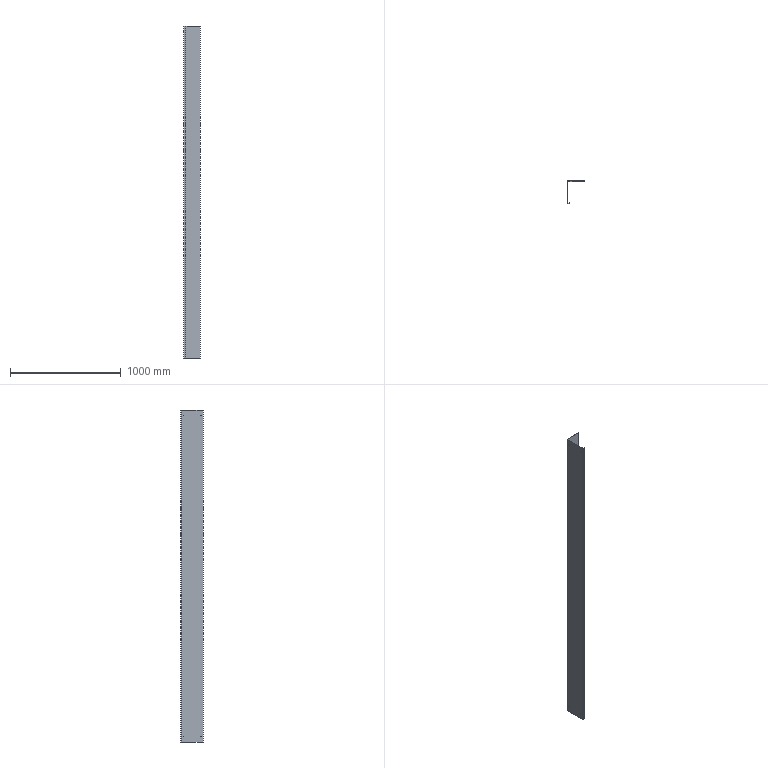Part | STEP file | TS-S19 | 1 solid | 30 faces | box 149.959 x 207.22 x 2995 mm | volume 2193923 mm3 | plane 18 | cylinder 12 | commonest cylinder face diameters 5.4 x8 0.4 x2 4.4 x2